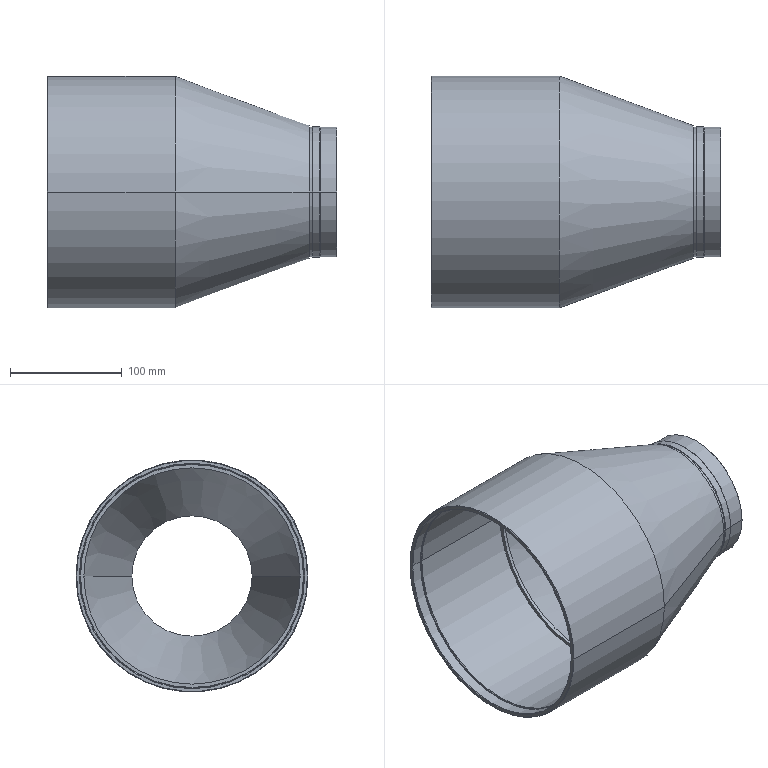Part | STEP file | lens barrel 1.stp.STEP-108.STEP | 1 solid | 44 faces | box 260 x 208 x 208 mm | volume 745018 mm3 | cone 18 | cylinder 18 | plane 8 | commonest cylinder face diameters 116 x4 108 x2 117 x2 194 x2 200 x2 201 x2
STEP:
#1=CARTESIAN_POINT('',(262.326,58.2,0.));
#2=VERTEX_POINT('',#1);
#3=CARTESIAN_POINT('',(262.326,-58.2,0.));
#4=VERTEX_POINT('',#3);
#5=CARTESIAN_POINT('',(262.326,0.,0.));
#6=DIRECTION('',(1.,0.,0.));
#7=DIRECTION('',(0.,1.,0.));
#8=AXIS2_PLACEMENT_3D('',#5,#6,#7);
#9=CIRCLE('',#8,58.2);
#10=EDGE_CURVE('',#2,#4,#9,.T.);
#11=ORIENTED_EDGE('',*,*,#10,.F.);
#12=CARTESIAN_POINT('',(262.026,58.5,0.));
#13=VERTEX_POINT('',#12);
#14=CARTESIAN_POINT('',(262.326,58.2,0.));
#15=DIRECTION('',(-0.7071,0.7071,0.));
#16=VECTOR('',#15,1000.);
#17=LINE('',#14,#16);
#18=EDGE_CURVE('',#2,#13,#17,.T.);
#19=ORIENTED_EDGE('',*,*,#18,.T.);
#20=CARTESIAN_POINT('',(262.026,-58.5,0.));
#21=VERTEX_POINT('',#20);
#22=CARTESIAN_POINT('',(262.026,0.,0.));
#23=DIRECTION('',(-1.,0.,0.));
#24=DIRECTION('',(0.,1.,0.));
#25=AXIS2_PLACEMENT_3D('',#22,#23,#24);
#26=CIRCLE('',#25,58.5);
#27=EDGE_CURVE('',#21,#13,#26,.T.);
#28=ORIENTED_EDGE('',*,*,#27,.F.);
#29=CARTESIAN_POINT('',(262.326,-58.2,0.));
#30=DIRECTION('',(-0.7071,-0.7071,0.));
#31=VECTOR('',#30,1000.);
#32=LINE('',#29,#31);
#33=EDGE_CURVE('',#4,#21,#32,.T.);
#34=ORIENTED_EDGE('',*,*,#33,.F.);
#35=EDGE_LOOP('',(#11,#19,#28,#34));
#36=FACE_OUTER_BOUND('',#35,.T.);
#37=CARTESIAN_POINT('',(262.326,0.,0.));
#38=DIRECTION('',(-1.,0.,0.));
#39=DIRECTION('',(0.,-1.,0.));
#40=AXIS2_PLACEMENT_3D('',#37,#38,#39);
#41=CONICAL_SURFACE('',#40,58.2,0.7854);
#42=ADVANCED_FACE('',(#36),#41,.T.);
#43=CARTESIAN_POINT('',(255.626,-58.5,0.));
#44=VERTEX_POINT('',#43);
#45=CARTESIAN_POINT('',(255.626,58.5,0.));
#46=VERTEX_POINT('',#45);
#47=CARTESIAN_POINT('',(255.626,0.,0.));
#48=DIRECTION('',(1.,0.,0.));
#49=DIRECTION('',(0.,-1.,0.));
#50=AXIS2_PLACEMENT_3D('',#47,#48,#49);
#51=CIRCLE('',#50,58.5);
#52=EDGE_CURVE('',#44,#46,#51,.T.);
#53=ORIENTED_EDGE('',*,*,#52,.T.);
#54=CARTESIAN_POINT('',(0.,58.5,0.));
#55=DIRECTION('',(1.,0.,0.));
#56=VECTOR('',#55,1000.);
#57=LINE('',#54,#56);
#58=EDGE_CURVE('',#46,#13,#57,.T.);
#59=ORIENTED_EDGE('',*,*,#58,.T.);
#60=CARTESIAN_POINT('',(262.026,0.,0.));
#61=DIRECTION('',(-1.,0.,0.));
#62=DIRECTION('',(0.,1.,0.));
#63=AXIS2_PLACEMENT_3D('',#60,#61,#62);
#64=CIRCLE('',#63,58.5);
#65=EDGE_CURVE('',#13,#21,#64,.T.);
#66=ORIENTED_EDGE('',*,*,#65,.T.);
#67=CARTESIAN_POINT('',(0.,-58.5,0.));
#68=DIRECTION('',(1.,0.,0.));
#69=VECTOR('',#68,1000.);
#70=LINE('',#67,#69);
#71=EDGE_CURVE('',#44,#21,#70,.T.);
#72=ORIENTED_EDGE('',*,*,#71,.F.);
#73=EDGE_LOOP('',(#53,#59,#66,#72));
#74=FACE_OUTER_BOUND('',#73,.T.);
#75=CARTESIAN_POINT('',(0.,0.,0.));
#76=DIRECTION('',(1.,0.,0.));
#77=DIRECTION('',(0.,-1.,0.));
#78=AXIS2_PLACEMENT_3D('',#75,#76,#77);
#79=CYLINDRICAL_SURFACE('',#78,58.5);
#80=ADVANCED_FACE('',(#74),#79,.T.);
#81=CARTESIAN_POINT('',(262.326,-58.,0.));
#82=VERTEX_POINT('',#81);
#83=CARTESIAN_POINT('',(262.326,58.,0.));
#84=VERTEX_POINT('',#83);
#85=CARTESIAN_POINT('',(262.326,0.,0.));
#86=DIRECTION('',(1.,0.,0.));
#87=DIRECTION('',(0.,-1.,0.));
#88=AXIS2_PLACEMENT_3D('',#85,#86,#87);
#89=CIRCLE('',#88,58.);
#90=EDGE_CURVE('',#82,#84,#89,.T.);
#91=ORIENTED_EDGE('',*,*,#90,.T.);
#92=CARTESIAN_POINT('',(276.826,58.,0.));
#93=VERTEX_POINT('',#92);
#94=CARTESIAN_POINT('',(0.,58.,0.));
#95=DIRECTION('',(1.,0.,0.));
#96=VECTOR('',#95,1000.);
#97=LINE('',#94,#96);
#98=EDGE_CURVE('',#84,#93,#97,.T.);
#99=ORIENTED_EDGE('',*,*,#98,.T.);
#100=CARTESIAN_POINT('',(276.826,-58.,0.));
#101=VERTEX_POINT('',#100);
#102=CARTESIAN_POINT('',(276.826,0.,0.));
#103=DIRECTION('',(-1.,0.,0.));
#104=DIRECTION('',(0.,1.,0.));
#105=AXIS2_PLACEMENT_3D('',#102,#103,#104);
#106=CIRCLE('',#105,58.);
#107=EDGE_CURVE('',#93,#101,#106,.T.);
#108=ORIENTED_EDGE('',*,*,#107,.T.);
#109=CARTESIAN_POINT('',(0.,-58.,0.));
#110=DIRECTION('',(1.,0.,0.));
#111=VECTOR('',#110,1000.);
#112=LINE('',#109,#111);
#113=EDGE_CURVE('',#82,#101,#112,.T.);
#114=ORIENTED_EDGE('',*,*,#113,.F.);
#115=EDGE_LOOP('',(#91,#99,#108,#114));
#116=FACE_OUTER_BOUND('',#115,.T.);
#117=CARTESIAN_POINT('',(0.,0.,0.));
#118=DIRECTION('',(1.,0.,0.));
#119=DIRECTION('',(0.,-1.,0.));
#120=AXIS2_PLACEMENT_3D('',#117,#118,#119);
#121=CYLINDRICAL_SURFACE('',#120,58.);
#122=ADVANCED_FACE('',(#116),#121,.T.);
#123=CARTESIAN_POINT('',(250.326,54.,0.));
#124=VERTEX_POINT('',#123);
#125=CARTESIAN_POINT('',(250.326,-54.,0.));
#126=VERTEX_POINT('',#125);
#127=CARTESIAN_POINT('',(250.326,0.,0.));
#128=DIRECTION('',(1.,0.,0.));
#129=DIRECTION('',(0.,-1.,0.));
#130=AXIS2_PLACEMENT_3D('',#127,#128,#129);
#131=CIRCLE('',#130,54.);
#132=EDGE_CURVE('',#124,#126,#131,.T.);
#133=ORIENTED_EDGE('',*,*,#132,.F.);
#134=CARTESIAN_POINT('',(276.826,54.,0.));
#135=VERTEX_POINT('',#134);
#136=CARTESIAN_POINT('',(0.,54.,0.));
#137=DIRECTION('',(1.,0.,0.));
#138=VECTOR('',#137,1000.);
#139=LINE('',#136,#138);
#140=EDGE_CURVE('',#124,#135,#139,.T.);
#141=ORIENTED_EDGE('',*,*,#140,.T.);
#142=CARTESIAN_POINT('',(276.826,-54.,0.));
#143=VERTEX_POINT('',#142);
#144=CARTESIAN_POINT('',(276.826,0.,0.));
#145=DIRECTION('',(1.,0.,0.));
#146=DIRECTION('',(0.,1.,0.));
#147=AXIS2_PLACEMENT_3D('',#144,#145,#146);
#148=CIRCLE('',#147,54.);
#149=EDGE_CURVE('',#135,#143,#148,.T.);
#150=ORIENTED_EDGE('',*,*,#149,.T.);
#151=CARTESIAN_POINT('',(0.,-54.,0.));
#152=DIRECTION('',(1.,0.,0.));
#153=VECTOR('',#152,1000.);
#154=LINE('',#151,#153);
#155=EDGE_CURVE('',#126,#143,#154,.T.);
#156=ORIENTED_EDGE('',*,*,#155,.F.);
#157=EDGE_LOOP('',(#133,#141,#150,#156));
#158=FACE_OUTER_BOUND('',#157,.T.);
#159=CARTESIAN_POINT('',(0.,0.,0.));
#160=DIRECTION('',(1.,0.,0.));
#161=DIRECTION('',(0.,-1.,0.));
#162=AXIS2_PLACEMENT_3D('',#159,#160,#161);
#163=CYLINDRICAL_SURFACE('',#162,54.);
#164=ADVANCED_FACE('',(#158),#163,.F.);
#165=CARTESIAN_POINT('',(276.826,0.,0.));
#166=DIRECTION('',(1.,0.,0.));
#167=DIRECTION('',(0.,1.,0.));
#168=AXIS2_PLACEMENT_3D('',#165,#166,#167);
#169=CIRCLE('',#168,54.);
#170=EDGE_CURVE('',#143,#135,#169,.T.);
#171=ORIENTED_EDGE('',*,*,#170,.F.);
#172=CARTESIAN_POINT('',(277.326,-54.5,0.));
#173=VERTEX_POINT('',#172);
#174=CARTESIAN_POINT('',(276.826,-54.,0.));
#175=DIRECTION('',(0.7071,-0.7071,0.));
#176=VECTOR('',#175,1000.);
#177=LINE('',#174,#176);
#178=EDGE_CURVE('',#143,#173,#177,.T.);
#179=ORIENTED_EDGE('',*,*,#178,.T.);
#180=CARTESIAN_POINT('',(277.326,54.5,0.));
#181=VERTEX_POINT('',#180);
#182=CARTESIAN_POINT('',(277.326,0.,0.));
#183=DIRECTION('',(-1.,0.,0.));
#184=DIRECTION('',(0.,1.,0.));
#185=AXIS2_PLACEMENT_3D('',#182,#183,#184);
#186=CIRCLE('',#185,54.5);
#187=EDGE_CURVE('',#181,#173,#186,.T.);
#188=ORIENTED_EDGE('',*,*,#187,.F.);
#189=CARTESIAN_POINT('',(276.826,54.,0.));
#190=DIRECTION('',(0.7071,0.7071,0.));
#191=VECTOR('',#190,1000.);
#192=LINE('',#189,#191);
#193=EDGE_CURVE('',#135,#181,#192,.T.);
#194=ORIENTED_EDGE('',*,*,#193,.F.);
#195=EDGE_LOOP('',(#171,#179,#188,#194));
#196=FACE_OUTER_BOUND('',#195,.T.);
#197=CARTESIAN_POINT('',(276.826,0.,0.));
#198=DIRECTION('',(1.,0.,0.));
#199=DIRECTION('',(0.,1.,0.));
#200=AXIS2_PLACEMENT_3D('',#197,#198,#199);
#201=CONICAL_SURFACE('',#200,54.,0.7854);
#202=ADVANCED_FACE('',(#196),#201,.F.);
#203=CARTESIAN_POINT('',(277.326,57.5,0.));
#204=VERTEX_POINT('',#203);
#205=CARTESIAN_POINT('',(277.326,-57.5,0.));
#206=VERTEX_POINT('',#205);
#207=CARTESIAN_POINT('',(277.326,0.,0.));
#208=DIRECTION('',(1.,0.,0.));
#209=DIRECTION('',(0.,1.,0.));
#210=AXIS2_PLACEMENT_3D('',#207,#208,#209);
#211=CIRCLE('',#210,57.5);
#212=EDGE_CURVE('',#204,#206,#211,.T.);
#213=ORIENTED_EDGE('',*,*,#212,.F.);
#214=CARTESIAN_POINT('',(277.326,57.5,0.));
#215=DIRECTION('',(-0.7071,0.7071,0.));
#216=VECTOR('',#215,1000.);
#217=LINE('',#214,#216);
#218=EDGE_CURVE('',#204,#93,#217,.T.);
#219=ORIENTED_EDGE('',*,*,#218,.T.);
#220=CARTESIAN_POINT('',(276.826,0.,0.));
#221=DIRECTION('',(-1.,0.,0.));
#222=DIRECTION('',(0.,1.,0.));
#223=AXIS2_PLACEMENT_3D('',#220,#221,#222);
#224=CIRCLE('',#223,58.);
#225=EDGE_CURVE('',#101,#93,#224,.T.);
#226=ORIENTED_EDGE('',*,*,#225,.F.);
#227=CARTESIAN_POINT('',(277.326,-57.5,0.));
#228=DIRECTION('',(-0.7071,-0.7071,0.));
#229=VECTOR('',#228,1000.);
#230=LINE('',#227,#229);
#231=EDGE_CURVE('',#206,#101,#230,.T.);
#232=ORIENTED_EDGE('',*,*,#231,.F.);
#233=EDGE_LOOP('',(#213,#219,#226,#232));
#234=FACE_OUTER_BOUND('',#233,.T.);
#235=CARTESIAN_POINT('',(277.326,0.,0.));
#236=DIRECTION('',(-1.,0.,0.));
#237=DIRECTION('',(0.,-1.,0.));
#238=AXIS2_PLACEMENT_3D('',#235,#236,#237);
#239=CONICAL_SURFACE('',#238,57.5,0.7854);
#240=ADVANCED_FACE('',(#234),#239,.T.);
#241=CARTESIAN_POINT('',(17.326,-103.5,0.));
#242=VERTEX_POINT('',#241);
#243=CARTESIAN_POINT('',(17.326,103.5,0.));
#244=VERTEX_POINT('',#243);
#245=CARTESIAN_POINT('',(17.326,0.,0.));
#246=DIRECTION('',(-1.,0.,0.));
#247=DIRECTION('',(0.,-1.,0.));
#248=AXIS2_PLACEMENT_3D('',#245,#246,#247);
#249=CIRCLE('',#248,103.5);
#250=EDGE_CURVE('',#242,#244,#249,.T.);
#251=ORIENTED_EDGE('',*,*,#250,.F.);
#252=CARTESIAN_POINT('',(17.826,-104.,0.));
#253=VERTEX_POINT('',#252);
#254=CARTESIAN_POINT('',(17.826,-104.,0.));
#255=DIRECTION('',(0.7071,-0.7071,0.));
#256=VECTOR('',#255,1000.);
#257=LINE('',#254,#256);
#258=EDGE_CURVE('',#242,#253,#257,.T.);
#259=ORIENTED_EDGE('',*,*,#258,.T.);
#260=CARTESIAN_POINT('',(17.826,104.,0.));
#261=VERTEX_POINT('',#260);
#262=CARTESIAN_POINT('',(17.826,0.,0.));
#263=DIRECTION('',(1.,0.,0.));
#264=DIRECTION('',(0.,-1.,0.));
#265=AXIS2_PLACEMENT_3D('',#262,#263,#264);
#266=CIRCLE('',#265,104.);
#267=EDGE_CURVE('',#261,#253,#266,.T.);
#268=ORIENTED_EDGE('',*,*,#267,.F.);
#269=CARTESIAN_POINT('',(17.826,104.,0.));
#270=DIRECTION('',(0.7071,0.7071,0.));
#271=VECTOR('',#270,1000.);
#272=LINE('',#269,#271);
#273=EDGE_CURVE('',#244,#261,#272,.T.);
#274=ORIENTED_EDGE('',*,*,#273,.F.);
#275=EDGE_LOOP('',(#251,#259,#268,#274));
#276=FACE_OUTER_BOUND('',#275,.T.);
#277=CARTESIAN_POINT('',(17.826,0.,0.));
#278=DIRECTION('',(1.,0.,0.));
#279=DIRECTION('',(0.,1.,0.));
#280=AXIS2_PLACEMENT_3D('',#277,#278,#279);
#281=CONICAL_SURFACE('',#280,104.,0.7854);
#282=ADVANCED_FACE('',(#276),#281,.T.);
#283=CARTESIAN_POINT('',(28.826,100.,0.));
#284=VERTEX_POINT('',#283);
#285=CARTESIAN_POINT('',(28.826,-100.,0.));
#286=VERTEX_POINT('',#285);
#287=CARTESIAN_POINT('',(28.826,0.,0.));
#288=DIRECTION('',(-1.,0.,0.));
#289=DIRECTION('',(0.,-1.,0.));
#290=AXIS2_PLACEMENT_3D('',#287,#288,#289);
#291=CIRCLE('',#290,100.);
#292=EDGE_CURVE('',#284,#286,#291,.T.);
#293=ORIENTED_EDGE('',*,*,#292,.F.);
#294=CARTESIAN_POINT('',(28.326,100.5,0.));
#295=VERTEX_POINT('',#294);
#296=CARTESIAN_POINT('',(28.326,100.5,0.));
#297=DIRECTION('',(-0.7071,0.7071,0.));
#298=VECTOR('',#297,1000.);
#299=LINE('',#296,#298);
#300=EDGE_CURVE('',#284,#295,#299,.T.);
#301=ORIENTED_EDGE('',*,*,#300,.T.);
#302=CARTESIAN_POINT('',(28.326,-100.5,0.));
#303=VERTEX_POINT('',#302);
#304=CARTESIAN_POINT('',(28.326,0.,0.));
#305=DIRECTION('',(1.,0.,0.));
#306=DIRECTION('',(0.,-1.,0.));
#307=AXIS2_PLACEMENT_3D('',#304,#305,#306);
#308=CIRCLE('',#307,100.5);
#309=EDGE_CURVE('',#303,#295,#308,.T.);
#310=ORIENTED_EDGE('',*,*,#309,.F.);
#311=CARTESIAN_POINT('',(28.326,-100.5,0.));
#312=DIRECTION('',(-0.7071,-0.7071,0.));
#313=VECTOR('',#312,1000.);
#314=LINE('',#311,#313);
#315=EDGE_CURVE('',#286,#303,#314,.T.);
#316=ORIENTED_EDGE('',*,*,#315,.F.);
#317=EDGE_LOOP('',(#293,#301,#310,#316));
#318=FACE_OUTER_BOUND('',#317,.T.);
#319=CARTESIAN_POINT('',(28.326,0.,0.));
#320=DIRECTION('',(-1.,0.,0.));
#321=DIRECTION('',(0.,-1.,0.));
#322=AXIS2_PLACEMENT_3D('',#319,#320,#321);
#323=CONICAL_SURFACE('',#322,100.5,0.7854);
#324=ADVANCED_FACE('',(#318),#323,.F.);
#325=CARTESIAN_POINT('',(17.826,100.5,0.));
#326=VERTEX_POINT('',#325);
#327=CARTESIAN_POINT('',(17.826,-100.5,0.));
#328=VERTEX_POINT('',#327);
#329=CARTESIAN_POINT('',(17.826,0.,0.));
#330=DIRECTION('',(-1.,0.,0.));
#331=DIRECTION('',(0.,-1.,0.));
#332=AXIS2_PLACEMENT_3D('',#329,#330,#331);
#333=CIRCLE('',#332,100.5);
#334=EDGE_CURVE('',#326,#328,#333,.T.);
#335=ORIENTED_EDGE('',*,*,#334,.F.);
#336=CARTESIAN_POINT('',(17.326,101.,0.));
#337=VERTEX_POINT('',#336);
#338=CARTESIAN_POINT('',(17.326,101.,0.));
#339=DIRECTION('',(-0.7071,0.7071,0.));
#340=VECTOR('',#339,1000.);
#341=LINE('',#338,#340);
#342=EDGE_CURVE('',#326,#337,#341,.T.);
#343=ORIENTED_EDGE('',*,*,#342,.T.);
#344=CARTESIAN_POINT('',(17.326,-101.,0.));
#345=VERTEX_POINT('',#344);
#346=CARTESIAN_POINT('',(17.326,0.,0.));
#347=DIRECTION('',(1.,0.,0.));
#348=DIRECTION('',(0.,-1.,0.));
#349=AXIS2_PLACEMENT_3D('',#346,#347,#348);
#350=CIRCLE('',#349,101.);
#351=EDGE_CURVE('',#345,#337,#350,.T.);
#352=ORIENTED_EDGE('',*,*,#351,.F.);
#353=CARTESIAN_POINT('',(17.326,-101.,0.));
#354=DIRECTION('',(-0.7071,-0.7071,0.));
#355=VECTOR('',#354,1000.);
#356=LINE('',#353,#355);
#357=EDGE_CURVE('',#328,#345,#356,.T.);
#358=ORIENTED_EDGE('',*,*,#357,.F.);
#359=EDGE_LOOP('',(#335,#343,#352,#358));
#360=FACE_OUTER_BOUND('',#359,.T.);
#361=CARTESIAN_POINT('',(17.326,0.,0.));
#362=DIRECTION('',(-1.,0.,0.));
#363=DIRECTION('',(0.,-1.,0.));
#364=AXIS2_PLACEMENT_3D('',#361,#362,#363);
#365=CONICAL_SURFACE('',#364,101.,0.7854);
#366=ADVANCED_FACE('',(#360),#365,.F.);
#367=CARTESIAN_POINT('',(17.826,0.,0.));
#368=DIRECTION('',(-1.,0.,0.));
#369=DIRECTION('',(0.,-1.,0.));
#370=AXIS2_PLACEMENT_3D('',#367,#368,#369);
#371=CIRCLE('',#370,100.5);
#372=EDGE_CURVE('',#328,#326,#371,.T.);
#373=ORIENTED_EDGE('',*,*,#372,.T.);
#374=CARTESIAN_POINT('',(27.326,100.5,0.));
#375=VERTEX_POINT('',#374);
#376=CARTESIAN_POINT('',(0.,100.5,0.));
#377=DIRECTION('',(1.,0.,0.));
#378=VECTOR('',#377,1000.);
#379=LINE('',#376,#378);
#380=EDGE_CURVE('',#326,#375,#379,.T.);
#381=ORIENTED_EDGE('',*,*,#380,.T.);
#382=CARTESIAN_POINT('',(27.326,-100.5,0.));
#383=VERTEX_POINT('',#382);
#384=CARTESIAN_POINT('',(27.326,0.,0.));
#385=DIRECTION('',(1.,0.,0.));
#386=DIRECTION('',(0.,-1.,0.));
#387=AXIS2_PLACEMENT_3D('',#384,#385,#386);
#388=CIRCLE('',#387,100.5);
#389=EDGE_CURVE('',#375,#383,#388,.T.);
#390=ORIENTED_EDGE('',*,*,#389,.T.);
#391=CARTESIAN_POINT('',(0.,-100.5,0.));
#392=DIRECTION('',(1.,0.,0.));
#393=VECTOR('',#392,1000.);
#394=LINE('',#391,#393);
#395=EDGE_CURVE('',#328,#383,#394,.T.);
#396=ORIENTED_EDGE('',*,*,#395,.F.);
#397=EDGE_LOOP('',(#373,#381,#390,#396));
#398=FACE_OUTER_BOUND('',#397,.T.);
#399=CARTESIAN_POINT('',(0.,0.,0.));
#400=DIRECTION('',(1.,0.,0.));
#401=DIRECTION('',(0.,-1.,0.));
#402=AXIS2_PLACEMENT_3D('',#399,#400,#401);
#403=CYLINDRICAL_SURFACE('',#402,100.5);
#404=ADVANCED_FACE('',(#398),#403,.F.);
#405=CARTESIAN_POINT('',(17.826,0.,0.));
#406=DIRECTION('',(1.,0.,0.));
#407=DIRECTION('',(0.,-1.,0.));
#408=AXIS2_PLACEMENT_3D('',#405,#406,#407);
#409=CIRCLE('',#408,104.);
#410=EDGE_CURVE('',#253,#261,#409,.T.);
#411=ORIENTED_EDGE('',*,*,#410,.T.);
#412=CARTESIAN_POINT('',(132.326,104.,0.));
#413=VERTEX_POINT('',#412);
#414=CARTESIAN_POINT('',(0.,104.,0.));
#415=DIRECTION('',(1.,0.,0.));
#416=VECTOR('',#415,1000.);
#417=LINE('',#414,#416);
#418=EDGE_CURVE('',#261,#413,#417,.T.);
#419=ORIENTED_EDGE('',*,*,#418,.T.);
#420=CARTESIAN_POINT('',(132.326,-104.,0.));
#421=VERTEX_POINT('',#420);
#422=CARTESIAN_POINT('',(132.326,0.,0.));
#423=DIRECTION('',(1.,0.,0.));
#424=DIRECTION('',(0.,-1.,0.));
#425=AXIS2_PLACEMENT_3D('',#422,#423,#424);
#426=CIRCLE('',#425,104.);
#427=EDGE_CURVE('',#421,#413,#426,.T.);
#428=ORIENTED_EDGE('',*,*,#427,.F.);
#429=CARTESIAN_POINT('',(0.,-104.,0.));
#430=DIRECTION('',(1.,0.,0.));
#431=VECTOR('',#430,1000.);
#432=LINE('',#429,#431);
#433=EDGE_CURVE('',#253,#421,#432,.T.);
#434=ORIENTED_EDGE('',*,*,#433,.F.);
#435=EDGE_LOOP('',(#411,#419,#428,#434));
#436=FACE_OUTER_BOUND('',#435,.T.);
#437=CARTESIAN_POINT('',(0.,0.,0.));
#438=DIRECTION('',(1.,0.,0.));
#439=DIRECTION('',(0.,-1.,0.));
#440=AXIS2_PLACEMENT_3D('',#437,#438,#439);
#441=CYLINDRICAL_SURFACE('',#440,104.);
#442=ADVANCED_FACE('',(#436),#441,.T.);
#443=CARTESIAN_POINT('',(252.326,-59.5,0.));
#444=VERTEX_POINT('',#443);
#445=CARTESIAN_POINT('',(252.326,59.5,0.));
#446=VERTEX_POINT('',#445);
#447=CARTESIAN_POINT('',(252.326,0.,0.));
#448=DIRECTION('',(1.,0.,0.));
#449=DIRECTION('',(0.,-1.,0.));
#450=AXIS2_PLACEMENT_3D('',#447,#448,#449);
#451=CIRCLE('',#450,59.5);
#452=EDGE_CURVE('',#444,#446,#451,.T.);
#453=ORIENTED_EDGE('',*,*,#452,.F.);
#454=CARTESIAN_POINT('',(252.326,-59.5,0.));
#455=DIRECTION('',(-0.9376,-0.3477,0.));
#456=VECTOR('',#455,1000.);
#457=LINE('',#454,#456);
#458=EDGE_CURVE('',#444,#421,#457,.T.);
#459=ORIENTED_EDGE('',*,*,#458,.T.);
#460=ORIENTED_EDGE('',*,*,#427,.T.);
#461=CARTESIAN_POINT('',(252.326,59.5,0.));
#462=DIRECTION('',(-0.9376,0.3477,0.));
#463=VECTOR('',#462,1000.);
#464=LINE('',#461,#463);
#465=EDGE_CURVE('',#446,#413,#464,.T.);
#466=ORIENTED_EDGE('',*,*,#465,.F.);
#467=EDGE_LOOP('',(#453,#459,#460,#466));
#468=FACE_OUTER_BOUND('',#467,.T.);
#469=CARTESIAN_POINT('',(252.326,0.,0.));
#470=DIRECTION('',(-1.,0.,0.));
#471=DIRECTION('',(0.,1.,0.));
#472=AXIS2_PLACEMENT_3D('',#469,#470,#471);
#473=CONICAL_SURFACE('',#472,59.5,0.3551);
#474=ADVANCED_FACE('',(#468),#473,.T.);
#475=CARTESIAN_POINT('',(252.326,-58.,0.));
#476=VERTEX_POINT('',#475);
#477=CARTESIAN_POINT('',(252.326,58.,0.));
#478=VERTEX_POINT('',#477);
#479=CARTESIAN_POINT('',(252.326,0.,0.));
#480=DIRECTION('',(1.,0.,0.));
#481=DIRECTION('',(0.,-1.,0.));
#482=AXIS2_PLACEMENT_3D('',#479,#480,#481);
#483=CIRCLE('',#482,58.);
#484=EDGE_CURVE('',#476,#478,#483,.T.);
#485=ORIENTED_EDGE('',*,*,#484,.T.);
#486=CARTESIAN_POINT('',(255.326,58.,0.));
#487=VERTEX_POINT('',#486);
#488=CARTESIAN_POINT('',(0.,58.,0.));
#489=DIRECTION('',(1.,0.,0.));
#490=VECTOR('',#489,1000.);
#491=LINE('',#488,#490);
#492=EDGE_CURVE('',#478,#487,#491,.T.);
#493=ORIENTED_EDGE('',*,*,#492,.T.);
#494=CARTESIAN_POINT('',(255.326,-58.,0.));
#495=VERTEX_POINT('',#494);
#496=CARTESIAN_POINT('',(255.326,0.,0.));
#497=DIRECTION('',(1.,0.,0.));
#498=DIRECTION('',(0.,-1.,0.));
#499=AXIS2_PLACEMENT_3D('',#496,#497,#498);
#500=CIRCLE('',#499,58.);
#501=EDGE_CURVE('',#495,#487,#500,.T.);
#502=ORIENTED_EDGE('',*,*,#501,.F.);
#503=CARTESIAN_POINT('',(0.,-58.,0.));
#504=DIRECTION('',(1.,0.,0.));
#505=VECTOR('',#504,1000.);
#506=LINE('',#503,#505);
#507=EDGE_CURVE('',#476,#495,#506,.T.);
#508=ORIENTED_EDGE('',*,*,#507,.F.);
#509=EDGE_LOOP('',(#485,#493,#502,#508));
#510=FACE_OUTER_BOUND('',#509,.T.);
#511=CARTESIAN_POINT('',(0.,0.,0.));
#512=DIRECTION('',(1.,0.,0.));
#513=DIRECTION('',(0.,-1.,0.));
#514=AXIS2_PLACEMENT_3D('',#511,#512,#513);
#515=CYLINDRICAL_SURFACE('',#514,58.);
#516=ADVANCED_FACE('',(#510),#515,.T.);
#517=CARTESIAN_POINT('',(28.826,0.,0.));
#518=DIRECTION('',(-1.,0.,0.));
#519=DIRECTION('',(0.,-1.,0.));
#520=AXIS2_PLACEMENT_3D('',#517,#518,#519);
#521=CIRCLE('',#520,100.);
#522=EDGE_CURVE('',#286,#284,#521,.T.);
#523=ORIENTED_EDGE('',*,*,#522,.T.);
#524=CARTESIAN_POINT('',(127.826,100.,0.));
#525=VERTEX_POINT('',#524);
#526=CARTESIAN_POINT('',(0.,100.,0.));
#527=DIRECTION('',(1.,0.,0.));
#528=VECTOR('',#527,1000.);
#529=LINE('',#526,#528);
#530=EDGE_CURVE('',#284,#525,#529,.T.);
#531=ORIENTED_EDGE('',*,*,#530,.T.);
#532=CARTESIAN_POINT('',(127.826,-100.,0.));
#533=VERTEX_POINT('',#532);
#534=CARTESIAN_POINT('',(127.826,0.,0.));
#535=DIRECTION('',(1.,0.,0.));
#536=DIRECTION('',(0.,-1.,0.));
#537=AXIS2_PLACEMENT_3D('',#534,#535,#536);
#538=CIRCLE('',#537,100.);
#539=EDGE_CURVE('',#525,#533,#538,.T.);
#540=ORIENTED_EDGE('',*,*,#539,.T.);
#541=CARTESIAN_POINT('',(0.,-100.,0.));
#542=DIRECTION('',(1.,0.,0.));
#543=VECTOR('',#542,1000.);
#544=LINE('',#541,#543);
#545=EDGE_CURVE('',#286,#533,#544,.T.);
#546=ORIENTED_EDGE('',*,*,#545,.F.);
#547=EDGE_LOOP('',(#523,#531,#540,#546));
#548=FACE_OUTER_BOUND('',#547,.T.);
#549=CARTESIAN_POINT('',(0.,0.,0.));
#550=DIRECTION('',(1.,0.,0.));
#551=DIRECTION('',(0.,-1.,0.));
#552=AXIS2_PLACEMENT_3D('',#549,#550,#551);
#553=CYLINDRICAL_SURFACE('',#552,100.);
#554=ADVANCED_FACE('',(#548),#553,.F.);
#555=CARTESIAN_POINT('',(27.326,101.5,0.));
#556=VERTEX_POINT('',#555);
#557=CARTESIAN_POINT('',(27.326,-101.5,0.));
#558=VERTEX_POINT('',#557);
#559=CARTESIAN_POINT('',(27.326,0.,0.));
#560=DIRECTION('',(1.,0.,0.));
#561=DIRECTION('',(0.,-1.,0.));
#562=AXIS2_PLACEMENT_3D('',#559,#560,#561);
#563=CIRCLE('',#562,101.5);
#564=EDGE_CURVE('',#556,#558,#563,.T.);
#565=ORIENTED_EDGE('',*,*,#564,.F.);
#566=CARTESIAN_POINT('',(28.326,101.5,0.));
#567=VERTEX_POINT('',#566);
#568=CARTESIAN_POINT('',(0.,101.5,0.));
#569=DIRECTION('',(1.,0.,0.));
#570=VECTOR('',#569,1000.);
#571=LINE('',#568,#570);
#572=EDGE_CURVE('',#556,#567,#571,.T.);
#573=ORIENTED_EDGE('',*,*,#572,.T.);
#574=CARTESIAN_POINT('',(28.326,-101.5,0.));
#575=VERTEX_POINT('',#574);
#576=CARTESIAN_POINT('',(28.326,0.,0.));
#577=DIRECTION('',(1.,0.,0.));
#578=DIRECTION('',(0.,-1.,0.));
#579=AXIS2_PLACEMENT_3D('',#576,#577,#578);
#580=CIRCLE('',#579,101.5);
#581=EDGE_CURVE('',#567,#575,#580,.T.);
#582=ORIENTED_EDGE('',*,*,#581,.T.);
#583=CARTESIAN_POINT('',(0.,-101.5,0.));
#584=DIRECTION('',(1.,0.,0.));
#585=VECTOR('',#584,1000.);
#586=LINE('',#583,#585);
#587=EDGE_CURVE('',#558,#575,#586,.T.);
#588=ORIENTED_EDGE('',*,*,#587,.F.);
#589=EDGE_LOOP('',(#565,#573,#582,#588));
#590=FACE_OUTER_BOUND('',#589,.T.);
#591=CARTESIAN_POINT('',(0.,0.,0.));
#592=DIRECTION('',(1.,0.,0.));
#593=DIRECTION('',(0.,-1.,0.));
#594=AXIS2_PLACEMENT_3D('',#591,#592,#593);
#595=CYLINDRICAL_SURFACE('',#594,101.5);
#596=ADVANCED_FACE('',(#590),#595,.F.);
#597=CARTESIAN_POINT('',(127.826,97.,0.));
#598=VERTEX_POINT('',#597);
#599=CARTESIAN_POINT('',(127.826,-97.,0.));
#600=VERTEX_POINT('',#599);
#601=CARTESIAN_POINT('',(127.826,0.,0.));
#602=DIRECTION('',(1.,0.,0.));
#603=DIRECTION('',(0.,-1.,0.));
#604=AXIS2_PLACEMENT_3D('',#601,#602,#603);
#605=CIRCLE('',#604,97.);
#606=EDGE_CURVE('',#598,#600,#605,.T.);
#607=ORIENTED_EDGE('',*,*,#606,.F.);
#608=CARTESIAN_POINT('',(130.826,97.,0.));
#609=VERTEX_POINT('',#608);
#610=CARTESIAN_POINT('',(0.,97.,0.));
#611=DIRECTION('',(1.,0.,0.));
#612=VECTOR('',#611,1000.);
#613=LINE('',#610,#612);
#614=EDGE_CURVE('',#598,#609,#613,.T.);
#615=ORIENTED_EDGE('',*,*,#614,.T.);
#616=CARTESIAN_POINT('',(130.826,-97.,0.));
#617=VERTEX_POINT('',#616);
#618=CARTESIAN_POINT('',(130.826,0.,0.));
#619=DIRECTION('',(1.,0.,0.));
#620=DIRECTION('',(0.,-1.,0.));
#621=AXIS2_PLACEMENT_3D('',#618,#619,#620);
#622=CIRCLE('',#621,97.);
#623=EDGE_CURVE('',#609,#617,#622,.T.);
#624=ORIENTED_EDGE('',*,*,#623,.T.);
#625=CARTESIAN_POINT('',(0.,-97.,0.));
#626=DIRECTION('',(1.,0.,0.));
#627=VECTOR('',#626,1000.);
#628=LINE('',#625,#627);
#629=EDGE_CURVE('',#600,#617,#628,.T.);
#630=ORIENTED_EDGE('',*,*,#629,.F.);
#631=EDGE_LOOP('',(#607,#615,#624,#630));
#632=FACE_OUTER_BOUND('',#631,.T.);
#633=CARTESIAN_POINT('',(0.,0.,0.));
#634=DIRECTION('',(1.,0.,0.));
#635=DIRECTION('',(0.,-1.,0.));
#636=AXIS2_PLACEMENT_3D('',#633,#634,#635);
#637=CYLINDRICAL_SURFACE('',#636,97.);
#638=ADVANCED_FACE('',(#632),#637,.F.);
#639=ORIENTED_EDGE('',*,*,#132,.T.);
#640=CARTESIAN_POINT('',(130.826,-97.,0.));
#641=DIRECTION('',(-0.9409,-0.3386,0.));
#642=VECTOR('',#641,1000.);
#643=LINE('',#640,#642);
#644=EDGE_CURVE('',#126,#617,#643,.T.);
#645=ORIENTED_EDGE('',*,*,#644,.T.);
#646=ORIENTED_EDGE('',*,*,#623,.F.);
#647=CARTESIAN_POINT('',(130.826,97.,0.));
#648=DIRECTION('',(-0.9409,0.3386,0.));
#649=VECTOR('',#648,1000.);
#650=LINE('',#647,#649);
#651=EDGE_CURVE('',#124,#609,#650,.T.);
#652=ORIENTED_EDGE('',*,*,#651,.F.);
#653=EDGE_LOOP('',(#639,#645,#646,#652));
#654=FACE_OUTER_BOUND('',#653,.T.);
#655=CARTESIAN_POINT('',(130.826,0.,0.));
#656=DIRECTION('',(-1.,0.,0.));
#657=DIRECTION('',(0.,1.,0.));
#658=AXIS2_PLACEMENT_3D('',#655,#656,#657);
#659=CONICAL_SURFACE('',#658,97.,0.3454);
#660=ADVANCED_FACE('',(#654),#659,.F.);
#661=CARTESIAN_POINT('',(255.326,-58.2,0.));
#662=VERTEX_POINT('',#661);
#663=CARTESIAN_POINT('',(255.326,58.2,0.));
#664=VERTEX_POINT('',#663);
#665=CARTESIAN_POINT('',(255.326,0.,0.));
#666=DIRECTION('',(-1.,0.,0.));
#667=DIRECTION('',(0.,-1.,0.));
#668=AXIS2_PLACEMENT_3D('',#665,#666,#667);
#669=CIRCLE('',#668,58.2);
#670=EDGE_CURVE('',#662,#664,#669,.T.);
#671=ORIENTED_EDGE('',*,*,#670,.F.);
#672=CARTESIAN_POINT('',(255.626,-58.5,0.));
#673=DIRECTION('',(0.7071,-0.7071,0.));
#674=VECTOR('',#673,1000.);
#675=LINE('',#672,#674);
#676=EDGE_CURVE('',#662,#44,#675,.T.);
#677=ORIENTED_EDGE('',*,*,#676,.T.);
#678=CARTESIAN_POINT('',(255.626,0.,0.));
#679=DIRECTION('',(1.,0.,0.));
#680=DIRECTION('',(0.,-1.,0.));
#681=AXIS2_PLACEMENT_3D('',#678,#679,#680);
#682=CIRCLE('',#681,58.5);
#683=EDGE_CURVE('',#46,#44,#682,.T.);
#684=ORIENTED_EDGE('',*,*,#683,.F.);
#685=CARTESIAN_POINT('',(255.626,58.5,0.));
#686=DIRECTION('',(0.7071,0.7071,0.));
#687=VECTOR('',#686,1000.);
#688=LINE('',#685,#687);
#689=EDGE_CURVE('',#664,#46,#688,.T.);
#690=ORIENTED_EDGE('',*,*,#689,.F.);
#691=EDGE_LOOP('',(#671,#677,#684,#690));
#692=FACE_OUTER_BOUND('',#691,.T.);
#693=CARTESIAN_POINT('',(255.626,0.,0.));
#694=DIRECTION('',(1.,0.,0.));
#695=DIRECTION('',(0.,1.,0.));
#696=AXIS2_PLACEMENT_3D('',#693,#694,#695);
#697=CONICAL_SURFACE('',#696,58.5,0.7854);
#698=ADVANCED_FACE('',(#692),#697,.T.);
#699=ORIENTED_EDGE('',*,*,#676,.F.);
#700=CARTESIAN_POINT('',(255.326,0.,0.));
#701=DIRECTION('',(-1.,0.,0.));
#702=DIRECTION('',(0.,-1.,0.));
#703=AXIS2_PLACEMENT_3D('',#700,#701,#702);
#704=CIRCLE('',#703,58.2);
#705=EDGE_CURVE('',#664,#662,#704,.T.);
#706=ORIENTED_EDGE('',*,*,#705,.F.);
#707=ORIENTED_EDGE('',*,*,#689,.T.);
#708=ORIENTED_EDGE('',*,*,#52,.F.);
#709=EDGE_LOOP('',(#699,#706,#707,#708));
#710=FACE_OUTER_BOUND('',#709,.T.);
#711=CARTESIAN_POINT('',(255.626,0.,0.));
#712=DIRECTION('',(1.,0.,0.));
#713=DIRECTION('',(0.,1.,0.));
#714=AXIS2_PLACEMENT_3D('',#711,#712,#713);
#715=CONICAL_SURFACE('',#714,58.5,0.7854);
#716=ADVANCED_FACE('',(#710),#715,.T.);
#717=ORIENTED_EDGE('',*,*,#644,.F.);
#718=CARTESIAN_POINT('',(250.326,0.,0.));
#719=DIRECTION('',(1.,0.,0.));
#720=DIRECTION('',(0.,-1.,0.));
#721=AXIS2_PLACEMENT_3D('',#718,#719,#720);
#722=CIRCLE('',#721,54.);
#723=EDGE_CURVE('',#126,#124,#722,.T.);
#724=ORIENTED_EDGE('',*,*,#723,.T.);
#725=ORIENTED_EDGE('',*,*,#651,.T.);
#726=CARTESIAN_POINT('',(130.826,0.,0.));
#727=DIRECTION('',(1.,0.,0.));
#728=DIRECTION('',(0.,-1.,0.));
#729=AXIS2_PLACEMENT_3D('',#726,#727,#728);
#730=CIRCLE('',#729,97.);
#731=EDGE_CURVE('',#617,#609,#730,.T.);
#732=ORIENTED_EDGE('',*,*,#731,.F.);
#733=EDGE_LOOP('',(#717,#724,#725,#732));
#734=FACE_OUTER_BOUND('',#733,.T.);
#735=CARTESIAN_POINT('',(130.826,0.,0.));
#736=DIRECTION('',(-1.,0.,0.));
#737=DIRECTION('',(0.,1.,0.));
#738=AXIS2_PLACEMENT_3D('',#735,#736,#737);
#739=CONICAL_SURFACE('',#738,97.,0.3454);
#740=ADVANCED_FACE('',(#734),#739,.F.);
#741=ORIENTED_EDGE('',*,*,#614,.F.);
#742=CARTESIAN_POINT('',(127.826,0.,0.));
#743=DIRECTION('',(1.,0.,0.));
#744=DIRECTION('',(0.,-1.,0.));
#745=AXIS2_PLACEMENT_3D('',#742,#743,#744);
#746=CIRCLE('',#745,97.);
#747=EDGE_CURVE('',#600,#598,#746,.T.);
#748=ORIENTED_EDGE('',*,*,#747,.F.);
#749=ORIENTED_EDGE('',*,*,#629,.T.);
#750=ORIENTED_EDGE('',*,*,#731,.T.);
#751=EDGE_LOOP('',(#741,#748,#749,#750));
#752=FACE_OUTER_BOUND('',#751,.T.);
#753=CARTESIAN_POINT('',(0.,0.,0.));
#754=DIRECTION('',(1.,0.,0.));
#755=DIRECTION('',(0.,-1.,0.));
#756=AXIS2_PLACEMENT_3D('',#753,#754,#755);
#757=CYLINDRICAL_SURFACE('',#756,97.);
#758=ADVANCED_FACE('',(#752),#757,.F.);
#759=ORIENTED_EDGE('',*,*,#747,.T.);
#760=ORIENTED_EDGE('',*,*,#606,.T.);
#761=EDGE_LOOP('',(#759,#760));
#762=FACE_BOUND('',#761,.T.);
#763=CARTESIAN_POINT('',(127.826,0.,0.));
#764=DIRECTION('',(1.,0.,0.));
#765=DIRECTION('',(0.,-1.,0.));
#766=AXIS2_PLACEMENT_3D('',#763,#764,#765);
#767=CIRCLE('',#766,100.);
#768=EDGE_CURVE('',#533,#525,#767,.T.);
#769=ORIENTED_EDGE('',*,*,#768,.F.);
#770=ORIENTED_EDGE('',*,*,#539,.F.);
#771=EDGE_LOOP('',(#769,#770));
#772=FACE_OUTER_BOUND('',#771,.T.);
#773=CARTESIAN_POINT('',(127.826,100.,0.));
#774=DIRECTION('',(-1.,0.,0.));
#775=DIRECTION('',(0.,1.,0.));
#776=AXIS2_PLACEMENT_3D('',#773,#774,#775);
#777=PLANE('',#776);
#778=ADVANCED_FACE('',(#762,#772),#777,.T.);
#779=CARTESIAN_POINT('',(27.326,0.,0.));
#780=DIRECTION('',(1.,0.,0.));
#781=DIRECTION('',(0.,-1.,0.));
#782=AXIS2_PLACEMENT_3D('',#779,#780,#781);
#783=CIRCLE('',#782,100.5);
#784=EDGE_CURVE('',#383,#375,#783,.T.);
#785=ORIENTED_EDGE('',*,*,#784,.F.);
#786=ORIENTED_EDGE('',*,*,#389,.F.);
#787=EDGE_LOOP('',(#785,#786));
#788=FACE_BOUND('',#787,.T.);
#789=CARTESIAN_POINT('',(27.326,0.,0.));
#790=DIRECTION('',(1.,0.,0.));
#791=DIRECTION('',(0.,-1.,0.));
#792=AXIS2_PLACEMENT_3D('',#789,#790,#791);
#793=CIRCLE('',#792,101.5);
#794=EDGE_CURVE('',#558,#556,#793,.T.);
#795=ORIENTED_EDGE('',*,*,#794,.T.);
#796=ORIENTED_EDGE('',*,*,#564,.T.);
#797=EDGE_LOOP('',(#795,#796));
#798=FACE_OUTER_BOUND('',#797,.T.);
#799=CARTESIAN_POINT('',(27.326,100.5,0.));
#800=DIRECTION('',(1.,0.,0.));
#801=DIRECTION('',(0.,1.,0.));
#802=AXIS2_PLACEMENT_3D('',#799,#800,#801);
#803=PLANE('',#802);
#804=ADVANCED_FACE('',(#788,#798),#803,.T.);
#805=ORIENTED_EDGE('',*,*,#572,.F.);
#806=ORIENTED_EDGE('',*,*,#794,.F.);
#807=ORIENTED_EDGE('',*,*,#587,.T.);
#808=CARTESIAN_POINT('',(28.326,0.,0.));
#809=DIRECTION('',(1.,0.,0.));
#810=DIRECTION('',(0.,-1.,0.));
#811=AXIS2_PLACEMENT_3D('',#808,#809,#810);
#812=CIRCLE('',#811,101.5);
#813=EDGE_CURVE('',#575,#567,#812,.T.);
#814=ORIENTED_EDGE('',*,*,#813,.T.);
#815=EDGE_LOOP('',(#805,#806,#807,#814));
#816=FACE_OUTER_BOUND('',#815,.T.);
#817=CARTESIAN_POINT('',(0.,0.,0.));
#818=DIRECTION('',(1.,0.,0.));
#819=DIRECTION('',(0.,-1.,0.));
#820=AXIS2_PLACEMENT_3D('',#817,#818,#819);
#821=CYLINDRICAL_SURFACE('',#820,101.5);
#822=ADVANCED_FACE('',(#816),#821,.F.);
#823=ORIENTED_EDGE('',*,*,#530,.F.);
#824=ORIENTED_EDGE('',*,*,#292,.T.);
#825=ORIENTED_EDGE('',*,*,#545,.T.);
#826=ORIENTED_EDGE('',*,*,#768,.T.);
#827=EDGE_LOOP('',(#823,#824,#825,#826));
#828=FACE_OUTER_BOUND('',#827,.T.);
#829=CARTESIAN_POINT('',(0.,0.,0.));
#830=DIRECTION('',(1.,0.,0.));
#831=DIRECTION('',(0.,-1.,0.));
#832=AXIS2_PLACEMENT_3D('',#829,#830,#831);
#833=CYLINDRICAL_SURFACE('',#832,100.);
#834=ADVANCED_FACE('',(#828),#833,.F.);
#835=ORIENTED_EDGE('',*,*,#309,.T.);
#836=CARTESIAN_POINT('',(28.326,0.,0.));
#837=DIRECTION('',(1.,0.,0.));
#838=DIRECTION('',(0.,-1.,0.));
#839=AXIS2_PLACEMENT_3D('',#836,#837,#838);
#840=CIRCLE('',#839,100.5);
#841=EDGE_CURVE('',#295,#303,#840,.T.);
#842=ORIENTED_EDGE('',*,*,#841,.T.);
#843=EDGE_LOOP('',(#835,#842));
#844=FACE_BOUND('',#843,.T.);
#845=ORIENTED_EDGE('',*,*,#813,.F.);
#846=ORIENTED_EDGE('',*,*,#581,.F.);
#847=EDGE_LOOP('',(#845,#846));
#848=FACE_OUTER_BOUND('',#847,.T.);
#849=CARTESIAN_POINT('',(28.326,101.5,0.));
#850=DIRECTION('',(-1.,0.,0.));
#851=DIRECTION('',(0.,1.,0.));
#852=AXIS2_PLACEMENT_3D('',#849,#850,#851);
#853=PLANE('',#852);
#854=ADVANCED_FACE('',(#844,#848),#853,.T.);
#855=ORIENTED_EDGE('',*,*,#501,.T.);
#856=CARTESIAN_POINT('',(255.326,0.,0.));
#857=DIRECTION('',(1.,0.,0.));
#858=DIRECTION('',(0.,-1.,0.));
#859=AXIS2_PLACEMENT_3D('',#856,#857,#858);
#860=CIRCLE('',#859,58.);
#861=EDGE_CURVE('',#487,#495,#860,.T.);
#862=ORIENTED_EDGE('',*,*,#861,.T.);
#863=EDGE_LOOP('',(#855,#862));
#864=FACE_BOUND('',#863,.T.);
#865=ORIENTED_EDGE('',*,*,#705,.T.);
#866=ORIENTED_EDGE('',*,*,#670,.T.);
#867=EDGE_LOOP('',(#865,#866));
#868=FACE_OUTER_BOUND('',#867,.T.);
#869=CARTESIAN_POINT('',(255.326,58.5,0.));
#870=DIRECTION('',(-1.,0.,0.));
#871=DIRECTION('',(0.,1.,0.));
#872=AXIS2_PLACEMENT_3D('',#869,#870,#871);
#873=PLANE('',#872);
#874=ADVANCED_FACE('',(#864,#868),#873,.T.);
#875=ORIENTED_EDGE('',*,*,#492,.F.);
#876=CARTESIAN_POINT('',(252.326,0.,0.));
#877=DIRECTION('',(1.,0.,0.));
#878=DIRECTION('',(0.,-1.,0.));
#879=AXIS2_PLACEMENT_3D('',#876,#877,#878);
#880=CIRCLE('',#879,58.);
#881=EDGE_CURVE('',#478,#476,#880,.T.);
#882=ORIENTED_EDGE('',*,*,#881,.T.);
#883=ORIENTED_EDGE('',*,*,#507,.T.);
#884=ORIENTED_EDGE('',*,*,#861,.F.);
#885=EDGE_LOOP('',(#875,#882,#883,#884));
#886=FACE_OUTER_BOUND('',#885,.T.);
#887=CARTESIAN_POINT('',(0.,0.,0.));
#888=DIRECTION('',(1.,0.,0.));
#889=DIRECTION('',(0.,-1.,0.));
#890=AXIS2_PLACEMENT_3D('',#887,#888,#889);
#891=CYLINDRICAL_SURFACE('',#890,58.);
#892=ADVANCED_FACE('',(#886),#891,.T.);
#893=ORIENTED_EDGE('',*,*,#484,.F.);
#894=ORIENTED_EDGE('',*,*,#881,.F.);
#895=EDGE_LOOP('',(#893,#894));
#896=FACE_BOUND('',#895,.T.);
#897=CARTESIAN_POINT('',(252.326,0.,0.));
#898=DIRECTION('',(1.,0.,0.));
#899=DIRECTION('',(0.,-1.,0.));
#900=AXIS2_PLACEMENT_3D('',#897,#898,#899);
#901=CIRCLE('',#900,59.5);
#902=EDGE_CURVE('',#446,#444,#901,.T.);
#903=ORIENTED_EDGE('',*,*,#902,.T.);
#904=ORIENTED_EDGE('',*,*,#452,.T.);
#905=EDGE_LOOP('',(#903,#904));
#906=FACE_OUTER_BOUND('',#905,.T.);
#907=CARTESIAN_POINT('',(252.326,58.,0.));
#908=DIRECTION('',(1.,0.,0.));
#909=DIRECTION('',(0.,1.,0.));
#910=AXIS2_PLACEMENT_3D('',#907,#908,#909);
#911=PLANE('',#910);
#912=ADVANCED_FACE('',(#896,#906),#911,.T.);
#913=ORIENTED_EDGE('',*,*,#458,.F.);
#914=ORIENTED_EDGE('',*,*,#902,.F.);
#915=ORIENTED_EDGE('',*,*,#465,.T.);
#916=CARTESIAN_POINT('',(132.326,0.,0.));
#917=DIRECTION('',(1.,0.,0.));
#918=DIRECTION('',(0.,-1.,0.));
#919=AXIS2_PLACEMENT_3D('',#916,#917,#918);
#920=CIRCLE('',#919,104.);
#921=EDGE_CURVE('',#413,#421,#920,.T.);
#922=ORIENTED_EDGE('',*,*,#921,.T.);
#923=EDGE_LOOP('',(#913,#914,#915,#922));
#924=FACE_OUTER_BOUND('',#923,.T.);
#925=CARTESIAN_POINT('',(252.326,0.,0.));
#926=DIRECTION('',(-1.,0.,0.));
#927=DIRECTION('',(0.,1.,0.));
#928=AXIS2_PLACEMENT_3D('',#925,#926,#927);
#929=CONICAL_SURFACE('',#928,59.5,0.3551);
#930=ADVANCED_FACE('',(#924),#929,.T.);
#931=ORIENTED_EDGE('',*,*,#418,.F.);
#932=ORIENTED_EDGE('',*,*,#267,.T.);
#933=ORIENTED_EDGE('',*,*,#433,.T.);
#934=ORIENTED_EDGE('',*,*,#921,.F.);
#935=EDGE_LOOP('',(#931,#932,#933,#934));
#936=FACE_OUTER_BOUND('',#935,.T.);
#937=CARTESIAN_POINT('',(0.,0.,0.));
#938=DIRECTION('',(1.,0.,0.));
#939=DIRECTION('',(0.,-1.,0.));
#940=AXIS2_PLACEMENT_3D('',#937,#938,#939);
#941=CYLINDRICAL_SURFACE('',#940,104.);
#942=ADVANCED_FACE('',(#936),#941,.T.);
#943=ORIENTED_EDGE('',*,*,#380,.F.);
#944=ORIENTED_EDGE('',*,*,#334,.T.);
#945=ORIENTED_EDGE('',*,*,#395,.T.);
#946=ORIENTED_EDGE('',*,*,#784,.T.);
#947=EDGE_LOOP('',(#943,#944,#945,#946));
#948=FACE_OUTER_BOUND('',#947,.T.);
#949=CARTESIAN_POINT('',(0.,0.,0.));
#950=DIRECTION('',(1.,0.,0.));
#951=DIRECTION('',(0.,-1.,0.));
#952=AXIS2_PLACEMENT_3D('',#949,#950,#951);
#953=CYLINDRICAL_SURFACE('',#952,100.5);
#954=ADVANCED_FACE('',(#948),#953,.F.);
#955=ORIENTED_EDGE('',*,*,#351,.T.);
#956=CARTESIAN_POINT('',(17.326,0.,0.));
#957=DIRECTION('',(1.,0.,0.));
#958=DIRECTION('',(0.,-1.,0.));
#959=AXIS2_PLACEMENT_3D('',#956,#957,#958);
#960=CIRCLE('',#959,101.);
#961=EDGE_CURVE('',#337,#345,#960,.T.);
#962=ORIENTED_EDGE('',*,*,#961,.T.);
#963=EDGE_LOOP('',(#955,#962));
#964=FACE_BOUND('',#963,.T.);
#965=CARTESIAN_POINT('',(17.326,0.,0.));
#966=DIRECTION('',(-1.,0.,0.));
#967=DIRECTION('',(0.,-1.,0.));
#968=AXIS2_PLACEMENT_3D('',#965,#966,#967);
#969=CIRCLE('',#968,103.5);
#970=EDGE_CURVE('',#244,#242,#969,.T.);
#971=ORIENTED_EDGE('',*,*,#970,.T.);
#972=ORIENTED_EDGE('',*,*,#250,.T.);
#973=EDGE_LOOP('',(#971,#972));
#974=FACE_OUTER_BOUND('',#973,.T.);
#975=CARTESIAN_POINT('',(17.326,104.,0.));
#976=DIRECTION('',(-1.,0.,0.));
#977=DIRECTION('',(0.,1.,0.));
#978=AXIS2_PLACEMENT_3D('',#975,#976,#977);
#979=PLANE('',#978);
#980=ADVANCED_FACE('',(#964,#974),#979,.T.);
#981=ORIENTED_EDGE('',*,*,#342,.F.);
#982=ORIENTED_EDGE('',*,*,#372,.F.);
#983=ORIENTED_EDGE('',*,*,#357,.T.);
#984=ORIENTED_EDGE('',*,*,#961,.F.);
#985=EDGE_LOOP('',(#981,#982,#983,#984));
#986=FACE_OUTER_BOUND('',#985,.T.);
#987=CARTESIAN_POINT('',(17.326,0.,0.));
#988=DIRECTION('',(-1.,0.,0.));
#989=DIRECTION('',(0.,-1.,0.));
#990=AXIS2_PLACEMENT_3D('',#987,#988,#989);
#991=CONICAL_SURFACE('',#990,101.,0.7854);
#992=ADVANCED_FACE('',(#986),#991,.F.);
#993=ORIENTED_EDGE('',*,*,#300,.F.);
#994=ORIENTED_EDGE('',*,*,#522,.F.);
#995=ORIENTED_EDGE('',*,*,#315,.T.);
#996=ORIENTED_EDGE('',*,*,#841,.F.);
#997=EDGE_LOOP('',(#993,#994,#995,#996));
#998=FACE_OUTER_BOUND('',#997,.T.);
#999=CARTESIAN_POINT('',(28.326,0.,0.));
#1000=DIRECTION('',(-1.,0.,0.));
#1001=DIRECTION('',(0.,-1.,0.));
#1002=AXIS2_PLACEMENT_3D('',#999,#1000,#1001);
#1003=CONICAL_SURFACE('',#1002,100.5,0.7854);
#1004=ADVANCED_FACE('',(#998),#1003,.F.);
#1005=ORIENTED_EDGE('',*,*,#258,.F.);
#1006=ORIENTED_EDGE('',*,*,#970,.F.);
#1007=ORIENTED_EDGE('',*,*,#273,.T.);
#1008=ORIENTED_EDGE('',*,*,#410,.F.);
#1009=EDGE_LOOP('',(#1005,#1006,#1007,#1008));
#1010=FACE_OUTER_BOUND('',#1009,.T.);
#1011=CARTESIAN_POINT('',(17.826,0.,0.));
#1012=DIRECTION('',(1.,0.,0.));
#1013=DIRECTION('',(0.,1.,0.));
#1014=AXIS2_PLACEMENT_3D('',#1011,#1012,#1013);
#1015=CONICAL_SURFACE('',#1014,104.,0.7854);
#1016=ADVANCED_FACE('',(#1010),#1015,.T.);
#1017=ORIENTED_EDGE('',*,*,#218,.F.);
#1018=CARTESIAN_POINT('',(277.326,0.,0.));
#1019=DIRECTION('',(1.,0.,0.));
#1020=DIRECTION('',(0.,1.,0.));
#1021=AXIS2_PLACEMENT_3D('',#1018,#1019,#1020);
#1022=CIRCLE('',#1021,57.5);
#1023=EDGE_CURVE('',#206,#204,#1022,.T.);
#1024=ORIENTED_EDGE('',*,*,#1023,.F.);
#1025=ORIENTED_EDGE('',*,*,#231,.T.);
#1026=ORIENTED_EDGE('',*,*,#107,.F.);
#1027=EDGE_LOOP('',(#1017,#1024,#1025,#1026));
#1028=FACE_OUTER_BOUND('',#1027,.T.);
#1029=CARTESIAN_POINT('',(277.326,0.,0.));
#1030=DIRECTION('',(-1.,0.,0.));
#1031=DIRECTION('',(0.,-1.,0.));
#1032=AXIS2_PLACEMENT_3D('',#1029,#1030,#1031);
#1033=CONICAL_SURFACE('',#1032,57.5,0.7854);
#1034=ADVANCED_FACE('',(#1028),#1033,.T.);
#1035=ORIENTED_EDGE('',*,*,#178,.F.);
#1036=ORIENTED_EDGE('',*,*,#149,.F.);
#1037=ORIENTED_EDGE('',*,*,#193,.T.);
#1038=CARTESIAN_POINT('',(277.326,0.,0.));
#1039=DIRECTION('',(-1.,0.,0.));
#1040=DIRECTION('',(0.,1.,0.));
#1041=AXIS2_PLACEMENT_3D('',#1038,#1039,#1040);
#1042=CIRCLE('',#1041,54.5);
#1043=EDGE_CURVE('',#173,#181,#1042,.T.);
#1044=ORIENTED_EDGE('',*,*,#1043,.F.);
#1045=EDGE_LOOP('',(#1035,#1036,#1037,#1044));
#1046=FACE_OUTER_BOUND('',#1045,.T.);
#1047=CARTESIAN_POINT('',(276.826,0.,0.));
#1048=DIRECTION('',(1.,0.,0.));
#1049=DIRECTION('',(0.,1.,0.));
#1050=AXIS2_PLACEMENT_3D('',#1047,#1048,#1049);
#1051=CONICAL_SURFACE('',#1050,54.,0.7854);
#1052=ADVANCED_FACE('',(#1046),#1051,.F.);
#1053=ORIENTED_EDGE('',*,*,#187,.T.);
#1054=ORIENTED_EDGE('',*,*,#1043,.T.);
#1055=EDGE_LOOP('',(#1053,#1054));
#1056=FACE_BOUND('',#1055,.T.);
#1057=ORIENTED_EDGE('',*,*,#1023,.T.);
#1058=ORIENTED_EDGE('',*,*,#212,.T.);
#1059=EDGE_LOOP('',(#1057,#1058));
#1060=FACE_OUTER_BOUND('',#1059,.T.);
#1061=CARTESIAN_POINT('',(277.326,54.,0.));
#1062=DIRECTION('',(1.,0.,0.));
#1063=DIRECTION('',(0.,1.,0.));
#1064=AXIS2_PLACEMENT_3D('',#1061,#1062,#1063);
#1065=PLANE('',#1064);
#1066=ADVANCED_FACE('',(#1056,#1060),#1065,.T.);
#1067=ORIENTED_EDGE('',*,*,#140,.F.);
#1068=ORIENTED_EDGE('',*,*,#723,.F.);
#1069=ORIENTED_EDGE('',*,*,#155,.T.);
#1070=ORIENTED_EDGE('',*,*,#170,.T.);
#1071=EDGE_LOOP('',(#1067,#1068,#1069,#1070));
#1072=FACE_OUTER_BOUND('',#1071,.T.);
#1073=CARTESIAN_POINT('',(0.,0.,0.));
#1074=DIRECTION('',(1.,0.,0.));
#1075=DIRECTION('',(0.,-1.,0.));
#1076=AXIS2_PLACEMENT_3D('',#1073,#1074,#1075);
#1077=CYLINDRICAL_SURFACE('',#1076,54.);
#1078=ADVANCED_FACE('',(#1072),#1077,.F.);
#1079=ORIENTED_EDGE('',*,*,#98,.F.);
#1080=CARTESIAN_POINT('',(262.326,0.,0.));
#1081=DIRECTION('',(1.,0.,0.));
#1082=DIRECTION('',(0.,-1.,0.));
#1083=AXIS2_PLACEMENT_3D('',#1080,#1081,#1082);
#1084=CIRCLE('',#1083,58.);
#1085=EDGE_CURVE('',#84,#82,#1084,.T.);
#1086=ORIENTED_EDGE('',*,*,#1085,.T.);
#1087=ORIENTED_EDGE('',*,*,#113,.T.);
#1088=ORIENTED_EDGE('',*,*,#225,.T.);
#1089=EDGE_LOOP('',(#1079,#1086,#1087,#1088));
#1090=FACE_OUTER_BOUND('',#1089,.T.);
#1091=CARTESIAN_POINT('',(0.,0.,0.));
#1092=DIRECTION('',(1.,0.,0.));
#1093=DIRECTION('',(0.,-1.,0.));
#1094=AXIS2_PLACEMENT_3D('',#1091,#1092,#1093);
#1095=CYLINDRICAL_SURFACE('',#1094,58.);
#1096=ADVANCED_FACE('',(#1090),#1095,.T.);
#1097=ORIENTED_EDGE('',*,*,#58,.F.);
#1098=ORIENTED_EDGE('',*,*,#683,.T.);
#1099=ORIENTED_EDGE('',*,*,#71,.T.);
#1100=ORIENTED_EDGE('',*,*,#27,.T.);
#1101=EDGE_LOOP('',(#1097,#1098,#1099,#1100));
#1102=FACE_OUTER_BOUND('',#1101,.T.);
#1103=CARTESIAN_POINT('',(0.,0.,0.));
#1104=DIRECTION('',(1.,0.,0.));
#1105=DIRECTION('',(0.,-1.,0.));
#1106=AXIS2_PLACEMENT_3D('',#1103,#1104,#1105);
#1107=CYLINDRICAL_SURFACE('',#1106,58.5);
#1108=ADVANCED_FACE('',(#1102),#1107,.T.);
#1109=ORIENTED_EDGE('',*,*,#90,.F.);
#1110=ORIENTED_EDGE('',*,*,#1085,.F.);
#1111=EDGE_LOOP('',(#1109,#1110));
#1112=FACE_BOUND('',#1111,.T.);
#1113=CARTESIAN_POINT('',(262.326,0.,0.));
#1114=DIRECTION('',(1.,0.,0.));
#1115=DIRECTION('',(0.,1.,0.));
#1116=AXIS2_PLACEMENT_3D('',#1113,#1114,#1115);
#1117=CIRCLE('',#1116,58.2);
#1118=EDGE_CURVE('',#4,#2,#1117,.T.);
#1119=ORIENTED_EDGE('',*,*,#1118,.T.);
#1120=ORIENTED_EDGE('',*,*,#10,.T.);
#1121=EDGE_LOOP('',(#1119,#1120));
#1122=FACE_OUTER_BOUND('',#1121,.T.);
#1123=CARTESIAN_POINT('',(262.326,58.,0.));
#1124=DIRECTION('',(1.,0.,0.));
#1125=DIRECTION('',(0.,1.,0.));
#1126=AXIS2_PLACEMENT_3D('',#1123,#1124,#1125);
#1127=PLANE('',#1126);
#1128=ADVANCED_FACE('',(#1112,#1122),#1127,.T.);
#1129=ORIENTED_EDGE('',*,*,#18,.F.);
#1130=ORIENTED_EDGE('',*,*,#1118,.F.);
#1131=ORIENTED_EDGE('',*,*,#33,.T.);
#1132=ORIENTED_EDGE('',*,*,#65,.F.);
#1133=EDGE_LOOP('',(#1129,#1130,#1131,#1132));
#1134=FACE_OUTER_BOUND('',#1133,.T.);
#1135=CARTESIAN_POINT('',(262.326,0.,0.));
#1136=DIRECTION('',(-1.,0.,0.));
#1137=DIRECTION('',(0.,-1.,0.));
#1138=AXIS2_PLACEMENT_3D('',#1135,#1136,#1137);
#1139=CONICAL_SURFACE('',#1138,58.2,0.7854);
#1140=ADVANCED_FACE('',(#1134),#1139,.T.);
#1141=CLOSED_SHELL('',(#42,#80,#122,#164,#202,#240,#282,#324,#366,#404,#442,#474,#516,#554,#596,#638,#660,#698,#716,#740,#758,#778,#804,#822,#834,#854,#874,#892,#912,#930,#942,#954,#980,#992,#1004,#1016,#1034,#1052,#1066,#1078,#1096,#1108,#1128,#1140));
#1142=MANIFOLD_SOLID_BREP('',#1141);
#1143=CARTESIAN_POINT('',(0.,0.,0.));
#1144=DIRECTION('',(0.,0.,1.));
#1145=DIRECTION('',(1.,0.,0.));
#1146=AXIS2_PLACEMENT_3D('',#1143,#1144,#1145);
#1147=(LENGTH_UNIT()NAMED_UNIT(*)SI_UNIT(.MILLI.,.METRE.));
#1148=UNCERTAINTY_MEASURE_WITH_UNIT(LENGTH_MEASURE(0.00001),#1147,'','');
#1149=(NAMED_UNIT(*)PLANE_ANGLE_UNIT()SI_UNIT($,.RADIAN.));
#1150=(NAMED_UNIT(*)SI_UNIT($,.STERADIAN.)SOLID_ANGLE_UNIT());
#1151=(GEOMETRIC_REPRESENTATION_CONTEXT(3)GLOBAL_UNCERTAINTY_ASSIGNED_CONTEXT((#1148))GLOBAL_UNIT_ASSIGNED_CONTEXT((#1147,#1149,#1150))REPRESENTATION_CONTEXT('',''));
#1152=ADVANCED_BREP_SHAPE_REPRESENTATION('',(#1142,#1146),#1151);